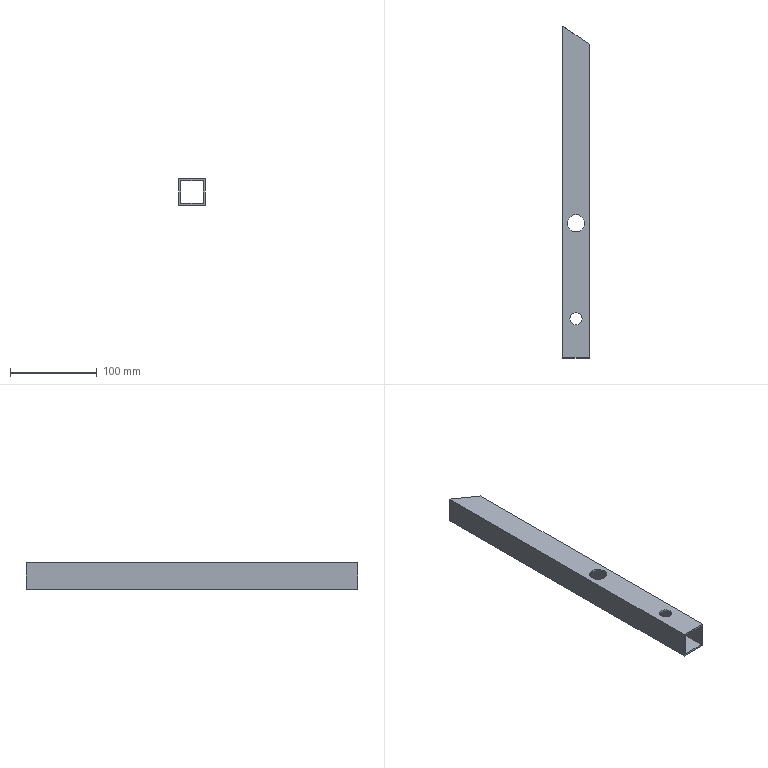Part | NX | features solid 2 | 1 solid | 14 faces | box 30 x 381.79 x 30 mm | volume 81296 mm3 | plane 10 | cylinder 4 | commonest cylinder face diameters 14 x2 20 x2
STEP:
#1=CARTESIAN_POINT('',(-430.,-14.216,-70.));
#2=VERTEX_POINT('',#1);
#3=CARTESIAN_POINT('',(-430.,-375.,-70.));
#4=VERTEX_POINT('',#3);
#5=CARTESIAN_POINT('',(-430.,-170.,-70.));
#6=DIRECTION('',(0.,-1.,0.));
#7=VECTOR('',#6,1000.);
#8=LINE('',#5,#7);
#9=EDGE_CURVE('',#2,#4,#8,.T.);
#10=ORIENTED_EDGE('',*,*,#9,.F.);
#11=CARTESIAN_POINT('',(-460.,6.79,-70.));
#12=VERTEX_POINT('',#11);
#13=CARTESIAN_POINT('',(-356.134,-65.937,-70.));
#14=DIRECTION('',(0.8192,-0.5736,0.));
#15=VECTOR('',#14,1000.);
#16=LINE('',#13,#15);
#17=EDGE_CURVE('',#2,#12,#16,.F.);
#18=ORIENTED_EDGE('',*,*,#17,.T.);
#19=CARTESIAN_POINT('',(-460.,-375.,-70.));
#20=VERTEX_POINT('',#19);
#21=CARTESIAN_POINT('',(-460.,-170.,-70.));
#22=DIRECTION('',(0.,1.,0.));
#23=VECTOR('',#22,1000.);
#24=LINE('',#21,#23);
#25=EDGE_CURVE('',#12,#20,#24,.F.);
#26=ORIENTED_EDGE('',*,*,#25,.T.);
#27=CARTESIAN_POINT('',(-429.,-375.,-70.));
#28=DIRECTION('',(-1.,0.,0.));
#29=VECTOR('',#28,1000.);
#30=LINE('',#27,#29);
#31=EDGE_CURVE('',#4,#20,#30,.T.);
#32=ORIENTED_EDGE('',*,*,#31,.F.);
#33=EDGE_LOOP('',(#10,#18,#26,#32));
#34=FACE_BOUND('',#33,.T.);
#35=CARTESIAN_POINT('',(-435.,-220.,-70.));
#36=VERTEX_POINT('',#35);
#37=CARTESIAN_POINT('',(-445.,-220.,-70.));
#38=DIRECTION('',(0.,0.,1.));
#39=DIRECTION('',(1.,0.,0.));
#40=AXIS2_PLACEMENT_3D('',#37,#38,#39);
#41=CIRCLE('',#40,10.);
#42=EDGE_CURVE('',#36,#36,#41,.F.);
#43=ORIENTED_EDGE('',*,*,#42,.T.);
#44=EDGE_LOOP('',(#43));
#45=FACE_BOUND('',#44,.T.);
#46=CARTESIAN_POINT('',(-438.,-330.,-70.));
#47=VERTEX_POINT('',#46);
#48=CARTESIAN_POINT('',(-445.,-330.,-70.));
#49=DIRECTION('',(0.,0.,1.));
#50=DIRECTION('',(1.,0.,0.));
#51=AXIS2_PLACEMENT_3D('',#48,#49,#50);
#52=CIRCLE('',#51,7.);
#53=EDGE_CURVE('',#47,#47,#52,.F.);
#54=ORIENTED_EDGE('',*,*,#53,.T.);
#55=EDGE_LOOP('',(#54));
#56=FACE_BOUND('',#55,.T.);
#57=CARTESIAN_POINT('',(-429.,-170.,-70.));
#58=DIRECTION('',(0.,0.,1.));
#59=DIRECTION('',(-1.,0.,0.));
#60=AXIS2_PLACEMENT_3D('',#57,#58,#59);
#61=PLANE('',#60);
#62=ADVANCED_FACE('',(#34,#45,#56),#61,.T.);
#63=CARTESIAN_POINT('',(-430.,-14.216,-100.));
#64=VERTEX_POINT('',#63);
#65=CARTESIAN_POINT('',(-460.,6.79,-100.));
#66=VERTEX_POINT('',#65);
#67=CARTESIAN_POINT('',(-356.134,-65.937,-100.));
#68=DIRECTION('',(0.8192,-0.5736,0.));
#69=VECTOR('',#68,1000.);
#70=LINE('',#67,#69);
#71=EDGE_CURVE('',#64,#66,#70,.F.);
#72=ORIENTED_EDGE('',*,*,#71,.F.);
#73=CARTESIAN_POINT('',(-430.,-375.,-100.));
#74=VERTEX_POINT('',#73);
#75=CARTESIAN_POINT('',(-430.,-170.,-100.));
#76=DIRECTION('',(0.,-1.,0.));
#77=VECTOR('',#76,1000.);
#78=LINE('',#75,#77);
#79=EDGE_CURVE('',#64,#74,#78,.T.);
#80=ORIENTED_EDGE('',*,*,#79,.T.);
#81=CARTESIAN_POINT('',(-460.,-375.,-100.));
#82=VERTEX_POINT('',#81);
#83=CARTESIAN_POINT('',(-429.,-375.,-100.));
#84=DIRECTION('',(-1.,0.,0.));
#85=VECTOR('',#84,1000.);
#86=LINE('',#83,#85);
#87=EDGE_CURVE('',#74,#82,#86,.T.);
#88=ORIENTED_EDGE('',*,*,#87,.T.);
#89=CARTESIAN_POINT('',(-460.,-170.,-100.));
#90=DIRECTION('',(0.,1.,0.));
#91=VECTOR('',#90,1000.);
#92=LINE('',#89,#91);
#93=EDGE_CURVE('',#66,#82,#92,.F.);
#94=ORIENTED_EDGE('',*,*,#93,.F.);
#95=EDGE_LOOP('',(#72,#80,#88,#94));
#96=FACE_BOUND('',#95,.T.);
#97=CARTESIAN_POINT('',(-435.,-220.,-100.));
#98=VERTEX_POINT('',#97);
#99=CARTESIAN_POINT('',(-445.,-220.,-100.));
#100=DIRECTION('',(0.,0.,1.));
#101=DIRECTION('',(1.,0.,0.));
#102=AXIS2_PLACEMENT_3D('',#99,#100,#101);
#103=CIRCLE('',#102,10.);
#104=EDGE_CURVE('',#98,#98,#103,.T.);
#105=ORIENTED_EDGE('',*,*,#104,.T.);
#106=EDGE_LOOP('',(#105));
#107=FACE_BOUND('',#106,.T.);
#108=CARTESIAN_POINT('',(-438.,-330.,-100.));
#109=VERTEX_POINT('',#108);
#110=CARTESIAN_POINT('',(-445.,-330.,-100.));
#111=DIRECTION('',(0.,0.,1.));
#112=DIRECTION('',(1.,0.,0.));
#113=AXIS2_PLACEMENT_3D('',#110,#111,#112);
#114=CIRCLE('',#113,7.);
#115=EDGE_CURVE('',#109,#109,#114,.T.);
#116=ORIENTED_EDGE('',*,*,#115,.T.);
#117=EDGE_LOOP('',(#116));
#118=FACE_BOUND('',#117,.T.);
#119=CARTESIAN_POINT('',(-429.,-170.,-100.));
#120=DIRECTION('',(0.,0.,1.));
#121=DIRECTION('',(-1.,0.,0.));
#122=AXIS2_PLACEMENT_3D('',#119,#120,#121);
#123=PLANE('',#122);
#124=ADVANCED_FACE('',(#96,#107,#118),#123,.F.);
#125=CARTESIAN_POINT('',(-458.,5.39,-98.));
#126=VERTEX_POINT('',#125);
#127=CARTESIAN_POINT('',(-432.,-12.815,-98.));
#128=VERTEX_POINT('',#127);
#129=CARTESIAN_POINT('',(-156.45,-205.758,-98.));
#130=DIRECTION('',(-0.8192,0.5736,0.));
#131=VECTOR('',#130,1000.);
#132=LINE('',#129,#131);
#133=EDGE_CURVE('',#126,#128,#132,.F.);
#134=ORIENTED_EDGE('',*,*,#133,.F.);
#135=CARTESIAN_POINT('',(-458.,-375.,-98.));
#136=VERTEX_POINT('',#135);
#137=CARTESIAN_POINT('',(-458.,-595.,-98.));
#138=DIRECTION('',(0.,1.,0.));
#139=VECTOR('',#138,1000.);
#140=LINE('',#137,#139);
#141=EDGE_CURVE('',#136,#126,#140,.T.);
#142=ORIENTED_EDGE('',*,*,#141,.F.);
#143=CARTESIAN_POINT('',(-432.,-375.,-98.));
#144=VERTEX_POINT('',#143);
#145=CARTESIAN_POINT('',(-280.472,-375.,-98.));
#146=DIRECTION('',(-1.,0.,0.));
#147=VECTOR('',#146,1000.);
#148=LINE('',#145,#147);
#149=EDGE_CURVE('',#144,#136,#148,.T.);
#150=ORIENTED_EDGE('',*,*,#149,.F.);
#151=CARTESIAN_POINT('',(-432.,-595.,-98.));
#152=DIRECTION('',(0.,1.,0.));
#153=VECTOR('',#152,1000.);
#154=LINE('',#151,#153);
#155=EDGE_CURVE('',#144,#128,#154,.T.);
#156=ORIENTED_EDGE('',*,*,#155,.T.);
#157=EDGE_LOOP('',(#134,#142,#150,#156));
#158=FACE_BOUND('',#157,.T.);
#159=CARTESIAN_POINT('',(-455.,-220.,-98.));
#160=VERTEX_POINT('',#159);
#161=CARTESIAN_POINT('',(-445.,-220.,-98.));
#162=DIRECTION('',(0.,0.,-1.));
#163=DIRECTION('',(-1.,0.,0.));
#164=AXIS2_PLACEMENT_3D('',#161,#162,#163);
#165=CIRCLE('',#164,10.);
#166=EDGE_CURVE('',#160,#160,#165,.T.);
#167=ORIENTED_EDGE('',*,*,#166,.T.);
#168=EDGE_LOOP('',(#167));
#169=FACE_BOUND('',#168,.T.);
#170=CARTESIAN_POINT('',(-452.,-330.,-98.));
#171=VERTEX_POINT('',#170);
#172=CARTESIAN_POINT('',(-445.,-330.,-98.));
#173=DIRECTION('',(0.,0.,-1.));
#174=DIRECTION('',(-1.,0.,0.));
#175=AXIS2_PLACEMENT_3D('',#172,#173,#174);
#176=CIRCLE('',#175,7.);
#177=EDGE_CURVE('',#171,#171,#176,.F.);
#178=ORIENTED_EDGE('',*,*,#177,.F.);
#179=EDGE_LOOP('',(#178));
#180=FACE_BOUND('',#179,.T.);
#181=CARTESIAN_POINT('',(-429.,-595.,-98.));
#182=DIRECTION('',(0.,0.,-1.));
#183=DIRECTION('',(1.,0.,0.));
#184=AXIS2_PLACEMENT_3D('',#181,#182,#183);
#185=PLANE('',#184);
#186=ADVANCED_FACE('',(#158,#169,#180),#185,.F.);
#187=CARTESIAN_POINT('',(-458.,-375.,-72.));
#188=VERTEX_POINT('',#187);
#189=CARTESIAN_POINT('',(-458.,5.39,-72.));
#190=VERTEX_POINT('',#189);
#191=CARTESIAN_POINT('',(-458.,-595.,-72.));
#192=DIRECTION('',(0.,1.,0.));
#193=VECTOR('',#192,1000.);
#194=LINE('',#191,#193);
#195=EDGE_CURVE('',#188,#190,#194,.T.);
#196=ORIENTED_EDGE('',*,*,#195,.T.);
#197=CARTESIAN_POINT('',(-432.,-12.815,-72.));
#198=VERTEX_POINT('',#197);
#199=CARTESIAN_POINT('',(-156.45,-205.758,-72.));
#200=DIRECTION('',(-0.8192,0.5736,0.));
#201=VECTOR('',#200,1000.);
#202=LINE('',#199,#201);
#203=EDGE_CURVE('',#190,#198,#202,.F.);
#204=ORIENTED_EDGE('',*,*,#203,.T.);
#205=CARTESIAN_POINT('',(-432.,-375.,-72.));
#206=VERTEX_POINT('',#205);
#207=CARTESIAN_POINT('',(-432.,-595.,-72.));
#208=DIRECTION('',(0.,1.,0.));
#209=VECTOR('',#208,1000.);
#210=LINE('',#207,#209);
#211=EDGE_CURVE('',#206,#198,#210,.T.);
#212=ORIENTED_EDGE('',*,*,#211,.F.);
#213=CARTESIAN_POINT('',(-280.472,-375.,-72.));
#214=DIRECTION('',(-1.,0.,0.));
#215=VECTOR('',#214,1000.);
#216=LINE('',#213,#215);
#217=EDGE_CURVE('',#206,#188,#216,.T.);
#218=ORIENTED_EDGE('',*,*,#217,.T.);
#219=EDGE_LOOP('',(#196,#204,#212,#218));
#220=FACE_BOUND('',#219,.T.);
#221=CARTESIAN_POINT('',(-455.,-220.,-72.));
#222=VERTEX_POINT('',#221);
#223=CARTESIAN_POINT('',(-445.,-220.,-72.));
#224=DIRECTION('',(0.,0.,-1.));
#225=DIRECTION('',(-1.,0.,0.));
#226=AXIS2_PLACEMENT_3D('',#223,#224,#225);
#227=CIRCLE('',#226,10.);
#228=EDGE_CURVE('',#222,#222,#227,.T.);
#229=ORIENTED_EDGE('',*,*,#228,.F.);
#230=EDGE_LOOP('',(#229));
#231=FACE_BOUND('',#230,.T.);
#232=CARTESIAN_POINT('',(-452.,-330.,-72.));
#233=VERTEX_POINT('',#232);
#234=CARTESIAN_POINT('',(-445.,-330.,-72.));
#235=DIRECTION('',(0.,0.,-1.));
#236=DIRECTION('',(-1.,0.,0.));
#237=AXIS2_PLACEMENT_3D('',#234,#235,#236);
#238=CIRCLE('',#237,7.);
#239=EDGE_CURVE('',#233,#233,#238,.F.);
#240=ORIENTED_EDGE('',*,*,#239,.T.);
#241=EDGE_LOOP('',(#240));
#242=FACE_BOUND('',#241,.T.);
#243=CARTESIAN_POINT('',(-429.,-595.,-72.));
#244=DIRECTION('',(0.,0.,-1.));
#245=DIRECTION('',(1.,0.,0.));
#246=AXIS2_PLACEMENT_3D('',#243,#244,#245);
#247=PLANE('',#246);
#248=ADVANCED_FACE('',(#220,#231,#242),#247,.T.);
#249=CARTESIAN_POINT('',(-460.,6.79,-95.));
#250=DIRECTION('',(0.,0.,1.));
#251=VECTOR('',#250,1000.);
#252=LINE('',#249,#251);
#253=EDGE_CURVE('',#66,#12,#252,.T.);
#254=ORIENTED_EDGE('',*,*,#253,.F.);
#255=ORIENTED_EDGE('',*,*,#93,.T.);
#256=CARTESIAN_POINT('',(-460.,-375.,-80.));
#257=DIRECTION('',(0.,0.,1.));
#258=VECTOR('',#257,1000.);
#259=LINE('',#256,#258);
#260=EDGE_CURVE('',#20,#82,#259,.F.);
#261=ORIENTED_EDGE('',*,*,#260,.F.);
#262=ORIENTED_EDGE('',*,*,#25,.F.);
#263=EDGE_LOOP('',(#254,#255,#261,#262));
#264=FACE_BOUND('',#263,.T.);
#265=CARTESIAN_POINT('',(-460.,-170.,-95.));
#266=DIRECTION('',(-1.,0.,0.));
#267=DIRECTION('',(0.,-1.,0.));
#268=AXIS2_PLACEMENT_3D('',#265,#266,#267);
#269=PLANE('',#268);
#270=ADVANCED_FACE('',(#264),#269,.T.);
#271=CARTESIAN_POINT('',(-430.,-14.216,-95.));
#272=DIRECTION('',(0.,0.,1.));
#273=VECTOR('',#272,1000.);
#274=LINE('',#271,#273);
#275=EDGE_CURVE('',#2,#64,#274,.F.);
#276=ORIENTED_EDGE('',*,*,#275,.F.);
#277=ORIENTED_EDGE('',*,*,#9,.T.);
#278=CARTESIAN_POINT('',(-430.,-375.,-95.));
#279=DIRECTION('',(0.,0.,-1.));
#280=VECTOR('',#279,1000.);
#281=LINE('',#278,#280);
#282=EDGE_CURVE('',#4,#74,#281,.T.);
#283=ORIENTED_EDGE('',*,*,#282,.T.);
#284=ORIENTED_EDGE('',*,*,#79,.F.);
#285=EDGE_LOOP('',(#276,#277,#283,#284));
#286=FACE_BOUND('',#285,.T.);
#287=CARTESIAN_POINT('',(-430.,-170.,-95.));
#288=DIRECTION('',(-1.,0.,0.));
#289=DIRECTION('',(0.,-1.,0.));
#290=AXIS2_PLACEMENT_3D('',#287,#288,#289);
#291=PLANE('',#290);
#292=ADVANCED_FACE('',(#286),#291,.F.);
#293=CARTESIAN_POINT('',(-432.,-12.815,-95.));
#294=DIRECTION('',(0.,0.,-1.));
#295=VECTOR('',#294,1000.);
#296=LINE('',#293,#295);
#297=EDGE_CURVE('',#128,#198,#296,.F.);
#298=ORIENTED_EDGE('',*,*,#297,.F.);
#299=ORIENTED_EDGE('',*,*,#155,.F.);
#300=CARTESIAN_POINT('',(-432.,-375.,-80.));
#301=DIRECTION('',(0.,0.,-1.));
#302=VECTOR('',#301,1000.);
#303=LINE('',#300,#302);
#304=EDGE_CURVE('',#206,#144,#303,.T.);
#305=ORIENTED_EDGE('',*,*,#304,.F.);
#306=ORIENTED_EDGE('',*,*,#211,.T.);
#307=EDGE_LOOP('',(#298,#299,#305,#306));
#308=FACE_BOUND('',#307,.T.);
#309=CARTESIAN_POINT('',(-432.,-595.,-95.));
#310=DIRECTION('',(1.,0.,0.));
#311=DIRECTION('',(0.,0.,1.));
#312=AXIS2_PLACEMENT_3D('',#309,#310,#311);
#313=PLANE('',#312);
#314=ADVANCED_FACE('',(#308),#313,.F.);
#315=ORIENTED_EDGE('',*,*,#141,.T.);
#316=CARTESIAN_POINT('',(-458.,5.39,-95.));
#317=DIRECTION('',(0.,0.,-1.));
#318=VECTOR('',#317,1000.);
#319=LINE('',#316,#318);
#320=EDGE_CURVE('',#126,#190,#319,.F.);
#321=ORIENTED_EDGE('',*,*,#320,.T.);
#322=ORIENTED_EDGE('',*,*,#195,.F.);
#323=CARTESIAN_POINT('',(-458.,-375.,-80.));
#324=DIRECTION('',(0.,0.,-1.));
#325=VECTOR('',#324,1000.);
#326=LINE('',#323,#325);
#327=EDGE_CURVE('',#188,#136,#326,.T.);
#328=ORIENTED_EDGE('',*,*,#327,.T.);
#329=EDGE_LOOP('',(#315,#321,#322,#328));
#330=FACE_BOUND('',#329,.T.);
#331=CARTESIAN_POINT('',(-458.,-595.,-95.));
#332=DIRECTION('',(1.,0.,0.));
#333=DIRECTION('',(0.,0.,1.));
#334=AXIS2_PLACEMENT_3D('',#331,#332,#333);
#335=PLANE('',#334);
#336=ADVANCED_FACE('',(#330),#335,.T.);
#337=ORIENTED_EDGE('',*,*,#42,.F.);
#338=EDGE_LOOP('',(#337));
#339=FACE_BOUND('',#338,.T.);
#340=ORIENTED_EDGE('',*,*,#228,.T.);
#341=EDGE_LOOP('',(#340));
#342=FACE_BOUND('',#341,.T.);
#343=CARTESIAN_POINT('',(-445.,-220.,-42.));
#344=DIRECTION('',(0.,0.,-1.));
#345=DIRECTION('',(1.,0.,0.));
#346=AXIS2_PLACEMENT_3D('',#343,#344,#345);
#347=CYLINDRICAL_SURFACE('',#346,10.);
#348=ADVANCED_FACE('',(#339,#342),#347,.F.);
#349=ORIENTED_EDGE('',*,*,#217,.F.);
#350=ORIENTED_EDGE('',*,*,#304,.T.);
#351=ORIENTED_EDGE('',*,*,#149,.T.);
#352=ORIENTED_EDGE('',*,*,#327,.F.);
#353=EDGE_LOOP('',(#349,#350,#351,#352));
#354=FACE_BOUND('',#353,.T.);
#355=ORIENTED_EDGE('',*,*,#260,.T.);
#356=ORIENTED_EDGE('',*,*,#87,.F.);
#357=ORIENTED_EDGE('',*,*,#282,.F.);
#358=ORIENTED_EDGE('',*,*,#31,.T.);
#359=EDGE_LOOP('',(#355,#356,#357,#358));
#360=FACE_BOUND('',#359,.T.);
#361=CARTESIAN_POINT('',(-280.472,-375.,-80.));
#362=DIRECTION('',(0.,1.,0.));
#363=DIRECTION('',(0.,0.,1.));
#364=AXIS2_PLACEMENT_3D('',#361,#362,#363);
#365=PLANE('',#364);
#366=ADVANCED_FACE('',(#354,#360),#365,.F.);
#367=ORIENTED_EDGE('',*,*,#166,.F.);
#368=EDGE_LOOP('',(#367));
#369=FACE_BOUND('',#368,.T.);
#370=ORIENTED_EDGE('',*,*,#104,.F.);
#371=EDGE_LOOP('',(#370));
#372=FACE_BOUND('',#371,.T.);
#373=CARTESIAN_POINT('',(-445.,-220.,-42.));
#374=DIRECTION('',(0.,0.,-1.));
#375=DIRECTION('',(1.,0.,0.));
#376=AXIS2_PLACEMENT_3D('',#373,#374,#375);
#377=CYLINDRICAL_SURFACE('',#376,10.);
#378=ADVANCED_FACE('',(#369,#372),#377,.F.);
#379=ORIENTED_EDGE('',*,*,#320,.F.);
#380=ORIENTED_EDGE('',*,*,#133,.T.);
#381=ORIENTED_EDGE('',*,*,#297,.T.);
#382=ORIENTED_EDGE('',*,*,#203,.F.);
#383=EDGE_LOOP('',(#379,#380,#381,#382));
#384=FACE_BOUND('',#383,.T.);
#385=ORIENTED_EDGE('',*,*,#71,.T.);
#386=ORIENTED_EDGE('',*,*,#253,.T.);
#387=ORIENTED_EDGE('',*,*,#17,.F.);
#388=ORIENTED_EDGE('',*,*,#275,.T.);
#389=EDGE_LOOP('',(#385,#386,#387,#388));
#390=FACE_BOUND('',#389,.T.);
#391=CARTESIAN_POINT('',(-526.263,53.188,-70.));
#392=DIRECTION('',(-0.5736,-0.8192,0.));
#393=DIRECTION('',(0.8192,-0.5736,0.));
#394=AXIS2_PLACEMENT_3D('',#391,#392,#393);
#395=PLANE('',#394);
#396=ADVANCED_FACE('',(#384,#390),#395,.F.);
#397=ORIENTED_EDGE('',*,*,#53,.F.);
#398=EDGE_LOOP('',(#397));
#399=FACE_BOUND('',#398,.T.);
#400=ORIENTED_EDGE('',*,*,#239,.F.);
#401=EDGE_LOOP('',(#400));
#402=FACE_BOUND('',#401,.T.);
#403=CARTESIAN_POINT('',(-445.,-330.,-95.));
#404=DIRECTION('',(0.,0.,-1.));
#405=DIRECTION('',(1.,0.,0.));
#406=AXIS2_PLACEMENT_3D('',#403,#404,#405);
#407=CYLINDRICAL_SURFACE('',#406,7.);
#408=ADVANCED_FACE('',(#399,#402),#407,.F.);
#409=ORIENTED_EDGE('',*,*,#115,.F.);
#410=EDGE_LOOP('',(#409));
#411=FACE_BOUND('',#410,.T.);
#412=ORIENTED_EDGE('',*,*,#177,.T.);
#413=EDGE_LOOP('',(#412));
#414=FACE_BOUND('',#413,.T.);
#415=CARTESIAN_POINT('',(-445.,-330.,-95.));
#416=DIRECTION('',(0.,0.,-1.));
#417=DIRECTION('',(1.,0.,0.));
#418=AXIS2_PLACEMENT_3D('',#415,#416,#417);
#419=CYLINDRICAL_SURFACE('',#418,7.);
#420=ADVANCED_FACE('',(#411,#414),#419,.F.);
#421=CLOSED_SHELL('',(#62,#124,#186,#248,#270,#292,#314,#336,#348,#366,#378,#396,#408,#420));
#422=MANIFOLD_SOLID_BREP('',#421);
#423=(LENGTH_UNIT()NAMED_UNIT(*)SI_UNIT(.MILLI.,.METRE.));
#424=UNCERTAINTY_MEASURE_WITH_UNIT(LENGTH_MEASURE(0.00001),#423,'','');
#425=(NAMED_UNIT(*)PLANE_ANGLE_UNIT()SI_UNIT($,.RADIAN.));
#426=(NAMED_UNIT(*)SI_UNIT($,.STERADIAN.)SOLID_ANGLE_UNIT());
#427=(GEOMETRIC_REPRESENTATION_CONTEXT(3)GLOBAL_UNCERTAINTY_ASSIGNED_CONTEXT((#424))GLOBAL_UNIT_ASSIGNED_CONTEXT((#423,#425,#426))REPRESENTATION_CONTEXT('',''));
#428=ADVANCED_BREP_SHAPE_REPRESENTATION('',(#422),#427);